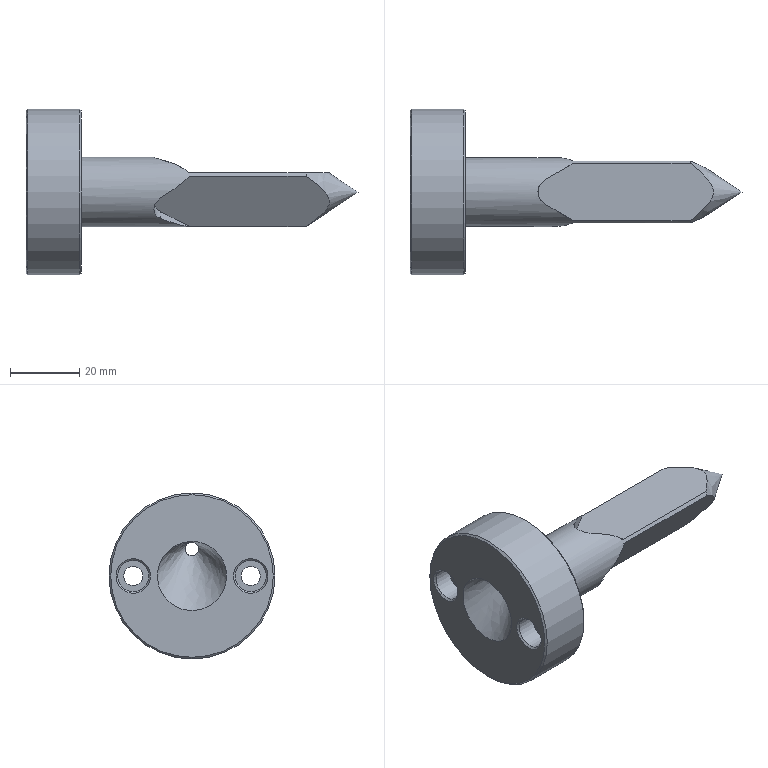CAM job | NX | 3+2 milling | part box 96 x 48 x 48 mm
Tools:
number,name,description,diameter,corner_radius,flute_length,length,flutes
8,D8,Milling Tool-5 Parameters,8.0,0.0,50.0,75.0,2
9,D8FINE,Milling Tool-5 Parameters,8.0,0.0,50.0,75.0,2
5,D3R0.5,Milling Tool-5 Parameters,3.0,0.5,50.0,75.0,2
Operations:
program,operation,operation_type,tool,method,geometry_group,spindle_rpm,surface_speed,feed_per_tooth,feed_cut,feed_plunge,cut_length_mm,path_length_mm,cut_time_min,machine_time_min
1-1,FLOOR_WALL,VolumeBased25DMillingOperation,D8,METHOD,A,3500.0,109.0,0.3143,2200.0,1001.0,4992.393,5407.126,2.353,2.394
1-1,FLOOR_WALL_COPY_1,VolumeBased25DMillingOperation,D8,METHOD,A,3500.0,109.0,0.3143,2200.0,1001.0,4992.393,5407.126,2.353,2.394
1-1,FLOOR_WALL_COPY_2,VolumeBased25DMillingOperation,D8,METHOD,A,3500.0,109.0,0.3143,2200.0,1001.0,4992.393,5407.126,2.353,2.394
1-2,FLOOR_WALL_COPY,VolumeBased25DMillingOperation,D8FINE,METHOD,A,5500.0,138.0,0.0909,1000.0,1001.0,385.692,479.237,0.3857,0.395
1-2,FLOOR_WALL_COPY_COPY,VolumeBased25DMillingOperation,D8FINE,METHOD,A,5500.0,138.0,0.0909,1000.0,1001.0,385.692,479.237,0.3857,0.395
1-2,FLOOR_WALL_COPY_COPY_1,VolumeBased25DMillingOperation,D8FINE,METHOD,A,5500.0,138.0,0.0909,1000.0,1001.0,385.692,479.237,0.3857,0.395
3,ZLEVEL_PROFILE,ZLevelMilling,D8,METHOD,B,3500.0,87.0,0.3143,2200.0,1000.0,1769.222,1834.516,0.8208,0.8273
3,ZLEVEL_PROFILE_COPY,ZLevelMilling,D3R0.5,METHOD,B,6500.0,61.0,0.1692,2200.0,1000.0,7272.902,7342.402,3.322,3.329